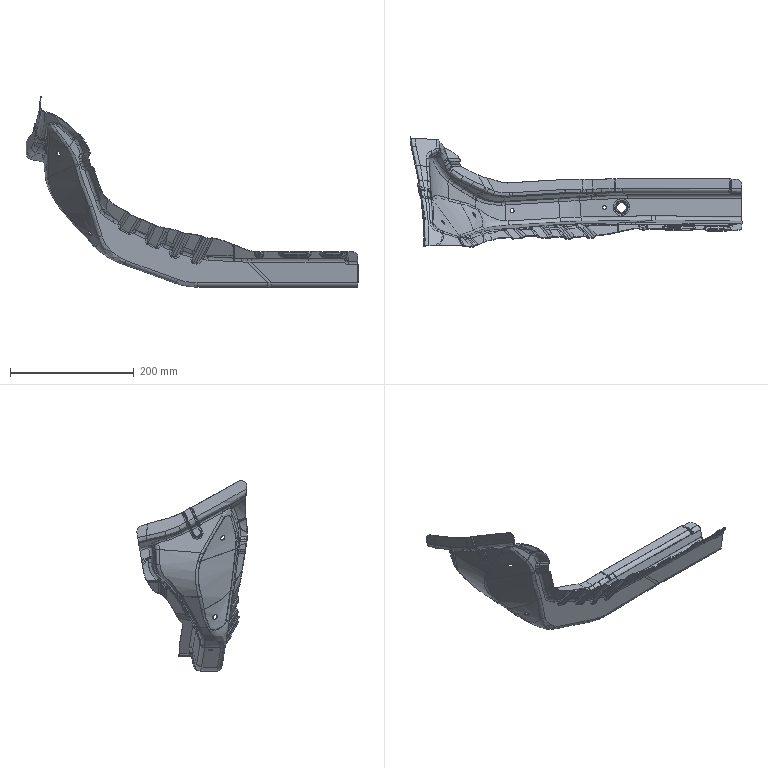Part | 1 solid | 949 faces | box 535.835 x 178.411 x 308.195 mm | volume 131485 mm3 | spline 711 | cylinder 147 | plane 71 | other 18 | sphere 2 | commonest cylinder face diameters 12 x18 10 x15 12.4 x11 13.6 x10 16 x10 9.6 x9